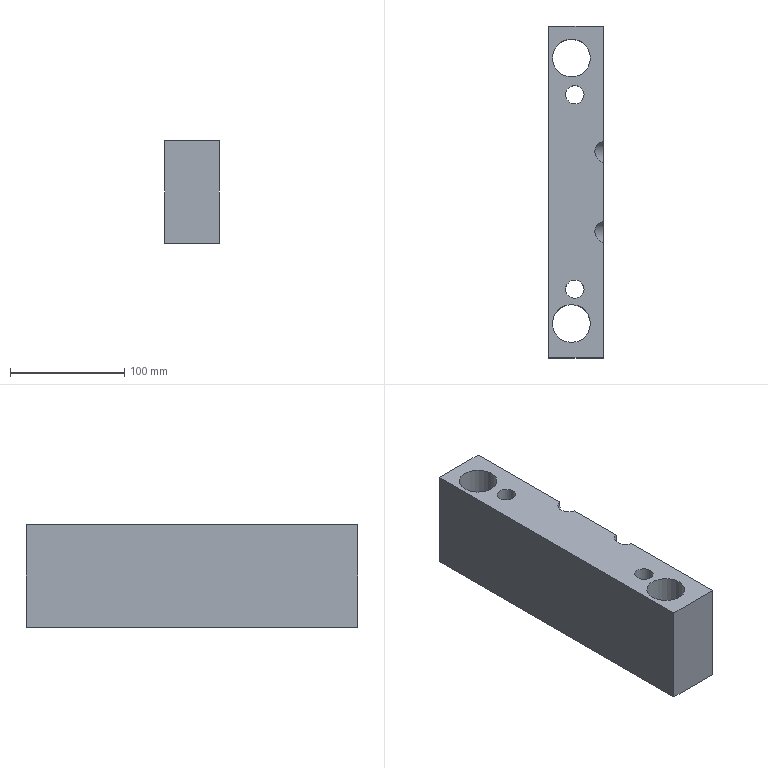Part | STEP file | CC02_id266_x_t | 1 solid | 18 faces | box 48 x 290 x 90 mm | volume 1057434 mm3 | plane 8 | cylinder 8 | cone 2 | commonest cylinder face diameters 10 x2 16 x2 20 x2 33 x2
STEP:
#1=CARTESIAN_POINT('',(113.5,117.,-165.5));
#2=VERTEX_POINT('',#1);
#3=CARTESIAN_POINT('',(97.,117.,-165.5));
#4=DIRECTION('',(0.,0.,1.));
#5=DIRECTION('',(1.,0.,0.));
#6=AXIS2_PLACEMENT_3D('',#3,#4,#5);
#7=CIRCLE('',#6,16.5);
#8=EDGE_CURVE('',#2,#2,#7,.T.);
#9=ORIENTED_EDGE('',*,*,#8,.T.);
#10=EDGE_LOOP('',(#9));
#11=FACE_BOUND('',#10,.T.);
#12=CARTESIAN_POINT('',(95.,-40.,-165.5));
#13=VERTEX_POINT('',#12);
#14=CARTESIAN_POINT('',(100.,-40.,-165.5));
#15=DIRECTION('',(0.,0.,1.));
#16=DIRECTION('',(-1.,0.,0.));
#17=AXIS2_PLACEMENT_3D('',#14,#15,#16);
#18=CIRCLE('',#17,5.);
#19=EDGE_CURVE('',#13,#13,#18,.T.);
#20=ORIENTED_EDGE('',*,*,#19,.T.);
#21=EDGE_LOOP('',(#20));
#22=FACE_BOUND('',#21,.T.);
#23=CARTESIAN_POINT('',(92.,-85.,-165.5));
#24=VERTEX_POINT('',#23);
#25=CARTESIAN_POINT('',(100.,-85.,-165.5));
#26=DIRECTION('',(0.,0.,1.));
#27=DIRECTION('',(-1.,0.,0.));
#28=AXIS2_PLACEMENT_3D('',#25,#26,#27);
#29=CIRCLE('',#28,8.);
#30=EDGE_CURVE('',#24,#24,#29,.T.);
#31=ORIENTED_EDGE('',*,*,#30,.T.);
#32=EDGE_LOOP('',(#31));
#33=FACE_BOUND('',#32,.T.);
#34=CARTESIAN_POINT('',(77.,145.,-165.5));
#35=VERTEX_POINT('',#34);
#36=CARTESIAN_POINT('',(77.,-145.,-165.5));
#37=VERTEX_POINT('',#36);
#38=CARTESIAN_POINT('',(77.,0.,-165.5));
#39=DIRECTION('',(0.,-1.,0.));
#40=VECTOR('',#39,1.);
#41=LINE('',#38,#40);
#42=EDGE_CURVE('',#35,#37,#41,.T.);
#43=ORIENTED_EDGE('',*,*,#42,.F.);
#44=CARTESIAN_POINT('',(125.,145.,-165.5));
#45=VERTEX_POINT('',#44);
#46=CARTESIAN_POINT('',(101.,145.,-165.5));
#47=DIRECTION('',(-1.,0.,0.));
#48=VECTOR('',#47,1.);
#49=LINE('',#46,#48);
#50=EDGE_CURVE('',#45,#35,#49,.T.);
#51=ORIENTED_EDGE('',*,*,#50,.F.);
#52=CARTESIAN_POINT('',(125.,-145.,-165.5));
#53=VERTEX_POINT('',#52);
#54=CARTESIAN_POINT('',(125.,0.,-165.5));
#55=DIRECTION('',(0.,1.,0.));
#56=VECTOR('',#55,1.);
#57=LINE('',#54,#56);
#58=EDGE_CURVE('',#53,#45,#57,.T.);
#59=ORIENTED_EDGE('',*,*,#58,.F.);
#60=CARTESIAN_POINT('',(101.,-145.,-165.5));
#61=DIRECTION('',(1.,0.,0.));
#62=VECTOR('',#61,1.);
#63=LINE('',#60,#62);
#64=EDGE_CURVE('',#37,#53,#63,.T.);
#65=ORIENTED_EDGE('',*,*,#64,.F.);
#66=EDGE_LOOP('',(#43,#51,#59,#65));
#67=FACE_BOUND('',#66,.T.);
#68=CARTESIAN_POINT('',(92.,85.,-165.5));
#69=VERTEX_POINT('',#68);
#70=CARTESIAN_POINT('',(100.,85.,-165.5));
#71=DIRECTION('',(0.,0.,1.));
#72=DIRECTION('',(-1.,0.,0.));
#73=AXIS2_PLACEMENT_3D('',#70,#71,#72);
#74=CIRCLE('',#73,8.);
#75=EDGE_CURVE('',#69,#69,#74,.T.);
#76=ORIENTED_EDGE('',*,*,#75,.T.);
#77=EDGE_LOOP('',(#76));
#78=FACE_BOUND('',#77,.T.);
#79=CARTESIAN_POINT('',(95.,40.,-165.5));
#80=VERTEX_POINT('',#79);
#81=CARTESIAN_POINT('',(100.,40.,-165.5));
#82=DIRECTION('',(0.,0.,1.));
#83=DIRECTION('',(-1.,0.,0.));
#84=AXIS2_PLACEMENT_3D('',#81,#82,#83);
#85=CIRCLE('',#84,5.);
#86=EDGE_CURVE('',#80,#80,#85,.T.);
#87=ORIENTED_EDGE('',*,*,#86,.T.);
#88=EDGE_LOOP('',(#87));
#89=FACE_BOUND('',#88,.T.);
#90=CARTESIAN_POINT('',(113.5,-115.,-165.5));
#91=VERTEX_POINT('',#90);
#92=CARTESIAN_POINT('',(97.,-115.,-165.5));
#93=DIRECTION('',(0.,0.,1.));
#94=DIRECTION('',(1.,0.,0.));
#95=AXIS2_PLACEMENT_3D('',#92,#93,#94);
#96=CIRCLE('',#95,16.5);
#97=EDGE_CURVE('',#91,#91,#96,.T.);
#98=ORIENTED_EDGE('',*,*,#97,.T.);
#99=EDGE_LOOP('',(#98));
#100=FACE_BOUND('',#99,.T.);
#101=CARTESIAN_POINT('',(101.,0.,-165.5));
#102=DIRECTION('',(0.,0.,-1.));
#103=DIRECTION('',(1.,0.,0.));
#104=AXIS2_PLACEMENT_3D('',#101,#102,#103);
#105=PLANE('',#104);
#106=ADVANCED_FACE('',(#11,#22,#33,#67,#78,#89,#100),#105,.T.);
#107=CARTESIAN_POINT('',(125.,-25.437,-75.5));
#108=VERTEX_POINT('',#107);
#109=CARTESIAN_POINT('',(125.,-44.563,-75.5));
#110=VERTEX_POINT('',#109);
#111=CARTESIAN_POINT('',(128.112,-35.,-75.5));
#112=DIRECTION('',(0.,0.,1.));
#113=DIRECTION('',(-1.,0.,0.));
#114=AXIS2_PLACEMENT_3D('',#111,#112,#113);
#115=ELLIPSE('',#114,10.642,10.);
#116=EDGE_CURVE('',#108,#110,#115,.T.);
#117=ORIENTED_EDGE('',*,*,#116,.F.);
#118=CARTESIAN_POINT('',(125.,25.437,-75.5));
#119=VERTEX_POINT('',#118);
#120=CARTESIAN_POINT('',(125.,0.,-75.5));
#121=DIRECTION('',(0.,-1.,0.));
#122=VECTOR('',#121,1.);
#123=LINE('',#120,#122);
#124=EDGE_CURVE('',#119,#108,#123,.T.);
#125=ORIENTED_EDGE('',*,*,#124,.F.);
#126=CARTESIAN_POINT('',(125.,44.563,-75.5));
#127=VERTEX_POINT('',#126);
#128=CARTESIAN_POINT('',(128.112,35.,-75.5));
#129=DIRECTION('',(0.,0.,1.));
#130=DIRECTION('',(-1.,0.,0.));
#131=AXIS2_PLACEMENT_3D('',#128,#129,#130);
#132=ELLIPSE('',#131,10.642,10.);
#133=EDGE_CURVE('',#127,#119,#132,.T.);
#134=ORIENTED_EDGE('',*,*,#133,.F.);
#135=CARTESIAN_POINT('',(125.,145.,-75.5));
#136=VERTEX_POINT('',#135);
#137=CARTESIAN_POINT('',(125.,0.,-75.5));
#138=DIRECTION('',(0.,-1.,0.));
#139=VECTOR('',#138,1.);
#140=LINE('',#137,#139);
#141=EDGE_CURVE('',#136,#127,#140,.T.);
#142=ORIENTED_EDGE('',*,*,#141,.F.);
#143=CARTESIAN_POINT('',(77.,145.,-75.5));
#144=VERTEX_POINT('',#143);
#145=CARTESIAN_POINT('',(101.,145.,-75.5));
#146=DIRECTION('',(1.,0.,0.));
#147=VECTOR('',#146,1.);
#148=LINE('',#145,#147);
#149=EDGE_CURVE('',#144,#136,#148,.T.);
#150=ORIENTED_EDGE('',*,*,#149,.F.);
#151=CARTESIAN_POINT('',(77.,-145.,-75.5));
#152=VERTEX_POINT('',#151);
#153=CARTESIAN_POINT('',(77.,0.,-75.5));
#154=DIRECTION('',(0.,1.,0.));
#155=VECTOR('',#154,1.);
#156=LINE('',#153,#155);
#157=EDGE_CURVE('',#152,#144,#156,.T.);
#158=ORIENTED_EDGE('',*,*,#157,.F.);
#159=CARTESIAN_POINT('',(125.,-145.,-75.5));
#160=VERTEX_POINT('',#159);
#161=CARTESIAN_POINT('',(101.,-145.,-75.5));
#162=DIRECTION('',(-1.,0.,0.));
#163=VECTOR('',#162,1.);
#164=LINE('',#161,#163);
#165=EDGE_CURVE('',#160,#152,#164,.T.);
#166=ORIENTED_EDGE('',*,*,#165,.F.);
#167=CARTESIAN_POINT('',(125.,0.,-75.5));
#168=DIRECTION('',(0.,-1.,0.));
#169=VECTOR('',#168,1.);
#170=LINE('',#167,#169);
#171=EDGE_CURVE('',#110,#160,#170,.T.);
#172=ORIENTED_EDGE('',*,*,#171,.F.);
#173=EDGE_LOOP('',(#117,#125,#134,#142,#150,#158,#166,#172));
#174=FACE_BOUND('',#173,.T.);
#175=CARTESIAN_POINT('',(113.5,117.,-75.5));
#176=VERTEX_POINT('',#175);
#177=CARTESIAN_POINT('',(97.,117.,-75.5));
#178=DIRECTION('',(0.,0.,-1.));
#179=DIRECTION('',(1.,0.,0.));
#180=AXIS2_PLACEMENT_3D('',#177,#178,#179);
#181=CIRCLE('',#180,16.5);
#182=EDGE_CURVE('',#176,#176,#181,.T.);
#183=ORIENTED_EDGE('',*,*,#182,.T.);
#184=EDGE_LOOP('',(#183));
#185=FACE_BOUND('',#184,.T.);
#186=CARTESIAN_POINT('',(108.,-85.,-75.5));
#187=VERTEX_POINT('',#186);
#188=CARTESIAN_POINT('',(100.,-85.,-75.5));
#189=DIRECTION('',(0.,0.,-1.));
#190=DIRECTION('',(1.,0.,0.));
#191=AXIS2_PLACEMENT_3D('',#188,#189,#190);
#192=CIRCLE('',#191,8.);
#193=EDGE_CURVE('',#187,#187,#192,.T.);
#194=ORIENTED_EDGE('',*,*,#193,.T.);
#195=EDGE_LOOP('',(#194));
#196=FACE_BOUND('',#195,.T.);
#197=CARTESIAN_POINT('',(108.,85.,-75.5));
#198=VERTEX_POINT('',#197);
#199=CARTESIAN_POINT('',(100.,85.,-75.5));
#200=DIRECTION('',(0.,0.,-1.));
#201=DIRECTION('',(1.,0.,0.));
#202=AXIS2_PLACEMENT_3D('',#199,#200,#201);
#203=CIRCLE('',#202,8.);
#204=EDGE_CURVE('',#198,#198,#203,.T.);
#205=ORIENTED_EDGE('',*,*,#204,.T.);
#206=EDGE_LOOP('',(#205));
#207=FACE_BOUND('',#206,.T.);
#208=CARTESIAN_POINT('',(113.5,-115.,-75.5));
#209=VERTEX_POINT('',#208);
#210=CARTESIAN_POINT('',(97.,-115.,-75.5));
#211=DIRECTION('',(0.,0.,-1.));
#212=DIRECTION('',(1.,0.,0.));
#213=AXIS2_PLACEMENT_3D('',#210,#211,#212);
#214=CIRCLE('',#213,16.5);
#215=EDGE_CURVE('',#209,#209,#214,.T.);
#216=ORIENTED_EDGE('',*,*,#215,.T.);
#217=EDGE_LOOP('',(#216));
#218=FACE_BOUND('',#217,.T.);
#219=CARTESIAN_POINT('',(101.,0.,-75.5));
#220=DIRECTION('',(0.,0.,1.));
#221=DIRECTION('',(-1.,0.,0.));
#222=AXIS2_PLACEMENT_3D('',#219,#220,#221);
#223=PLANE('',#222);
#224=ADVANCED_FACE('',(#174,#185,#196,#207,#218),#223,.T.);
#225=CARTESIAN_POINT('',(77.,145.,-165.5));
#226=DIRECTION('',(0.,0.,1.));
#227=VECTOR('',#226,1.);
#228=LINE('',#225,#227);
#229=EDGE_CURVE('',#35,#144,#228,.T.);
#230=ORIENTED_EDGE('',*,*,#229,.T.);
#231=ORIENTED_EDGE('',*,*,#149,.T.);
#232=CARTESIAN_POINT('',(125.,145.,-165.5));
#233=DIRECTION('',(0.,0.,1.));
#234=VECTOR('',#233,1.);
#235=LINE('',#232,#234);
#236=EDGE_CURVE('',#45,#136,#235,.T.);
#237=ORIENTED_EDGE('',*,*,#236,.F.);
#238=ORIENTED_EDGE('',*,*,#50,.T.);
#239=EDGE_LOOP('',(#230,#231,#237,#238));
#240=FACE_OUTER_BOUND('',#239,.T.);
#241=CARTESIAN_POINT('',(101.,145.,-165.5));
#242=DIRECTION('',(0.,1.,0.));
#243=DIRECTION('',(0.,0.,-1.));
#244=AXIS2_PLACEMENT_3D('',#241,#242,#243);
#245=PLANE('',#244);
#246=ADVANCED_FACE('',(#240),#245,.T.);
#247=CARTESIAN_POINT('',(125.,-35.,-66.95));
#248=DIRECTION('',(1.,0.,0.));
#249=DIRECTION('',(0.,0.,1.));
#250=AXIS2_PLACEMENT_3D('',#247,#248,#249);
#251=ELLIPSE('',#250,29.238,10.);
#252=EDGE_CURVE('',#110,#108,#251,.T.);
#253=ORIENTED_EDGE('',*,*,#252,.F.);
#254=ORIENTED_EDGE('',*,*,#171,.T.);
#255=CARTESIAN_POINT('',(125.,-145.,-165.5));
#256=DIRECTION('',(0.,0.,1.));
#257=VECTOR('',#256,1.);
#258=LINE('',#255,#257);
#259=EDGE_CURVE('',#53,#160,#258,.T.);
#260=ORIENTED_EDGE('',*,*,#259,.F.);
#261=ORIENTED_EDGE('',*,*,#58,.T.);
#262=ORIENTED_EDGE('',*,*,#236,.T.);
#263=ORIENTED_EDGE('',*,*,#141,.T.);
#264=CARTESIAN_POINT('',(125.,35.,-66.95));
#265=DIRECTION('',(1.,0.,0.));
#266=DIRECTION('',(0.,0.,1.));
#267=AXIS2_PLACEMENT_3D('',#264,#265,#266);
#268=ELLIPSE('',#267,29.238,10.);
#269=EDGE_CURVE('',#119,#127,#268,.T.);
#270=ORIENTED_EDGE('',*,*,#269,.F.);
#271=ORIENTED_EDGE('',*,*,#124,.T.);
#272=EDGE_LOOP('',(#253,#254,#260,#261,#262,#263,#270,#271));
#273=FACE_OUTER_BOUND('',#272,.T.);
#274=CARTESIAN_POINT('',(125.,0.,-165.5));
#275=DIRECTION('',(1.,0.,0.));
#276=DIRECTION('',(0.,0.,1.));
#277=AXIS2_PLACEMENT_3D('',#274,#275,#276);
#278=PLANE('',#277);
#279=ADVANCED_FACE('',(#273),#278,.T.);
#280=ORIENTED_EDGE('',*,*,#259,.T.);
#281=ORIENTED_EDGE('',*,*,#165,.T.);
#282=CARTESIAN_POINT('',(77.,-145.,-165.5));
#283=DIRECTION('',(0.,0.,1.));
#284=VECTOR('',#283,1.);
#285=LINE('',#282,#284);
#286=EDGE_CURVE('',#37,#152,#285,.T.);
#287=ORIENTED_EDGE('',*,*,#286,.F.);
#288=ORIENTED_EDGE('',*,*,#64,.T.);
#289=EDGE_LOOP('',(#280,#281,#287,#288));
#290=FACE_OUTER_BOUND('',#289,.T.);
#291=CARTESIAN_POINT('',(101.,-145.,-165.5));
#292=DIRECTION('',(0.,-1.,0.));
#293=DIRECTION('',(0.,0.,1.));
#294=AXIS2_PLACEMENT_3D('',#291,#292,#293);
#295=PLANE('',#294);
#296=ADVANCED_FACE('',(#290),#295,.T.);
#297=ORIENTED_EDGE('',*,*,#42,.T.);
#298=ORIENTED_EDGE('',*,*,#286,.T.);
#299=ORIENTED_EDGE('',*,*,#157,.T.);
#300=ORIENTED_EDGE('',*,*,#229,.F.);
#301=EDGE_LOOP('',(#297,#298,#299,#300));
#302=FACE_OUTER_BOUND('',#301,.T.);
#303=CARTESIAN_POINT('',(77.,0.,-165.5));
#304=DIRECTION('',(-1.,0.,0.));
#305=DIRECTION('',(0.,0.,-1.));
#306=AXIS2_PLACEMENT_3D('',#303,#304,#305);
#307=PLANE('',#306);
#308=ADVANCED_FACE('',(#302),#307,.T.);
#309=ORIENTED_EDGE('',*,*,#193,.F.);
#310=EDGE_LOOP('',(#309));
#311=FACE_BOUND('',#310,.T.);
#312=ORIENTED_EDGE('',*,*,#30,.F.);
#313=EDGE_LOOP('',(#312));
#314=FACE_BOUND('',#313,.T.);
#315=CARTESIAN_POINT('',(100.,-85.,-165.5));
#316=DIRECTION('',(0.,0.,1.));
#317=DIRECTION('',(-1.,0.,0.));
#318=AXIS2_PLACEMENT_3D('',#315,#316,#317);
#319=CYLINDRICAL_SURFACE('',#318,8.);
#320=ADVANCED_FACE('',(#311,#314),#319,.F.);
#321=ORIENTED_EDGE('',*,*,#204,.F.);
#322=EDGE_LOOP('',(#321));
#323=FACE_BOUND('',#322,.T.);
#324=ORIENTED_EDGE('',*,*,#75,.F.);
#325=EDGE_LOOP('',(#324));
#326=FACE_BOUND('',#325,.T.);
#327=CARTESIAN_POINT('',(100.,85.,-165.5));
#328=DIRECTION('',(0.,0.,1.));
#329=DIRECTION('',(-1.,0.,0.));
#330=AXIS2_PLACEMENT_3D('',#327,#328,#329);
#331=CYLINDRICAL_SURFACE('',#330,8.);
#332=ADVANCED_FACE('',(#323,#326),#331,.F.);
#333=CARTESIAN_POINT('',(95.5,-40.,-144.5));
#334=VERTEX_POINT('',#333);
#335=CARTESIAN_POINT('',(100.,-40.,-144.5));
#336=DIRECTION('',(0.,0.,1.));
#337=DIRECTION('',(-1.,0.,0.));
#338=AXIS2_PLACEMENT_3D('',#335,#336,#337);
#339=CIRCLE('',#338,4.5);
#340=EDGE_CURVE('',#334,#334,#339,.T.);
#341=ORIENTED_EDGE('',*,*,#340,.T.);
#342=EDGE_LOOP('',(#341));
#343=FACE_BOUND('',#342,.T.);
#344=CARTESIAN_POINT('',(105.,-40.,-144.5));
#345=VERTEX_POINT('',#344);
#346=CARTESIAN_POINT('',(100.,-40.,-144.5));
#347=DIRECTION('',(0.,0.,-1.));
#348=DIRECTION('',(1.,0.,0.));
#349=AXIS2_PLACEMENT_3D('',#346,#347,#348);
#350=CIRCLE('',#349,5.);
#351=EDGE_CURVE('',#345,#345,#350,.T.);
#352=ORIENTED_EDGE('',*,*,#351,.T.);
#353=EDGE_LOOP('',(#352));
#354=FACE_BOUND('',#353,.T.);
#355=CARTESIAN_POINT('',(100.,-40.,-144.5));
#356=DIRECTION('',(0.,0.,1.));
#357=DIRECTION('',(-1.,0.,0.));
#358=AXIS2_PLACEMENT_3D('',#355,#356,#357);
#359=PLANE('',#358);
#360=ADVANCED_FACE('',(#343,#354),#359,.F.);
#361=ORIENTED_EDGE('',*,*,#351,.F.);
#362=EDGE_LOOP('',(#361));
#363=FACE_BOUND('',#362,.T.);
#364=ORIENTED_EDGE('',*,*,#19,.F.);
#365=EDGE_LOOP('',(#364));
#366=FACE_BOUND('',#365,.T.);
#367=CARTESIAN_POINT('',(100.,-40.,-165.5));
#368=DIRECTION('',(0.,0.,1.));
#369=DIRECTION('',(-1.,0.,0.));
#370=AXIS2_PLACEMENT_3D('',#367,#368,#369);
#371=CYLINDRICAL_SURFACE('',#370,5.);
#372=ADVANCED_FACE('',(#363,#366),#371,.F.);
#373=CARTESIAN_POINT('',(95.5,40.,-144.5));
#374=VERTEX_POINT('',#373);
#375=CARTESIAN_POINT('',(100.,40.,-144.5));
#376=DIRECTION('',(0.,0.,1.));
#377=DIRECTION('',(-1.,0.,0.));
#378=AXIS2_PLACEMENT_3D('',#375,#376,#377);
#379=CIRCLE('',#378,4.5);
#380=EDGE_CURVE('',#374,#374,#379,.T.);
#381=ORIENTED_EDGE('',*,*,#380,.T.);
#382=EDGE_LOOP('',(#381));
#383=FACE_BOUND('',#382,.T.);
#384=CARTESIAN_POINT('',(105.,40.,-144.5));
#385=VERTEX_POINT('',#384);
#386=CARTESIAN_POINT('',(100.,40.,-144.5));
#387=DIRECTION('',(0.,0.,-1.));
#388=DIRECTION('',(1.,0.,0.));
#389=AXIS2_PLACEMENT_3D('',#386,#387,#388);
#390=CIRCLE('',#389,5.);
#391=EDGE_CURVE('',#385,#385,#390,.T.);
#392=ORIENTED_EDGE('',*,*,#391,.T.);
#393=EDGE_LOOP('',(#392));
#394=FACE_BOUND('',#393,.T.);
#395=CARTESIAN_POINT('',(100.,40.,-144.5));
#396=DIRECTION('',(0.,0.,1.));
#397=DIRECTION('',(-1.,0.,0.));
#398=AXIS2_PLACEMENT_3D('',#395,#396,#397);
#399=PLANE('',#398);
#400=ADVANCED_FACE('',(#383,#394),#399,.F.);
#401=ORIENTED_EDGE('',*,*,#391,.F.);
#402=EDGE_LOOP('',(#401));
#403=FACE_BOUND('',#402,.T.);
#404=ORIENTED_EDGE('',*,*,#86,.F.);
#405=EDGE_LOOP('',(#404));
#406=FACE_BOUND('',#405,.T.);
#407=CARTESIAN_POINT('',(100.,40.,-165.5));
#408=DIRECTION('',(0.,0.,1.));
#409=DIRECTION('',(-1.,0.,0.));
#410=AXIS2_PLACEMENT_3D('',#407,#408,#409);
#411=CYLINDRICAL_SURFACE('',#410,5.);
#412=ADVANCED_FACE('',(#403,#406),#411,.F.);
#413=ORIENTED_EDGE('',*,*,#340,.F.);
#414=EDGE_LOOP('',(#413));
#415=FACE_BOUND('',#414,.T.);
#416=CARTESIAN_POINT('',(100.,-40.,-142.05));
#417=VERTEX_POINT('',#416);
#418=VERTEX_LOOP('',#417);
#419=FACE_BOUND('',#418,.T.);
#420=CARTESIAN_POINT('',(100.,-40.,-142.05));
#421=DIRECTION('',(0.,0.,-1.));
#422=DIRECTION('',(1.,0.,0.));
#423=AXIS2_PLACEMENT_3D('',#420,#421,#422);
#424=CONICAL_SURFACE('',#423,0.,61.434);
#425=ADVANCED_FACE('',(#415,#419),#424,.F.);
#426=ORIENTED_EDGE('',*,*,#380,.F.);
#427=EDGE_LOOP('',(#426));
#428=FACE_BOUND('',#427,.T.);
#429=CARTESIAN_POINT('',(100.,40.,-142.05));
#430=VERTEX_POINT('',#429);
#431=VERTEX_LOOP('',#430);
#432=FACE_BOUND('',#431,.T.);
#433=CARTESIAN_POINT('',(100.,40.,-142.05));
#434=DIRECTION('',(0.,0.,-1.));
#435=DIRECTION('',(1.,0.,0.));
#436=AXIS2_PLACEMENT_3D('',#433,#434,#435);
#437=CONICAL_SURFACE('',#436,0.,61.434);
#438=ADVANCED_FACE('',(#428,#432),#437,.F.);
#439=ORIENTED_EDGE('',*,*,#182,.F.);
#440=EDGE_LOOP('',(#439));
#441=FACE_BOUND('',#440,.T.);
#442=ORIENTED_EDGE('',*,*,#8,.F.);
#443=EDGE_LOOP('',(#442));
#444=FACE_BOUND('',#443,.T.);
#445=CARTESIAN_POINT('',(97.,117.,-165.5));
#446=DIRECTION('',(0.,0.,1.));
#447=DIRECTION('',(1.,0.,0.));
#448=AXIS2_PLACEMENT_3D('',#445,#446,#447);
#449=CYLINDRICAL_SURFACE('',#448,16.5);
#450=ADVANCED_FACE('',(#441,#444),#449,.F.);
#451=ORIENTED_EDGE('',*,*,#215,.F.);
#452=EDGE_LOOP('',(#451));
#453=FACE_BOUND('',#452,.T.);
#454=ORIENTED_EDGE('',*,*,#97,.F.);
#455=EDGE_LOOP('',(#454));
#456=FACE_BOUND('',#455,.T.);
#457=CARTESIAN_POINT('',(97.,-115.,-165.5));
#458=DIRECTION('',(0.,0.,1.));
#459=DIRECTION('',(1.,0.,0.));
#460=AXIS2_PLACEMENT_3D('',#457,#458,#459);
#461=CYLINDRICAL_SURFACE('',#460,16.5);
#462=ADVANCED_FACE('',(#453,#456),#461,.F.);
#463=ORIENTED_EDGE('',*,*,#133,.T.);
#464=ORIENTED_EDGE('',*,*,#269,.T.);
#465=EDGE_LOOP('',(#463,#464));
#466=FACE_OUTER_BOUND('',#465,.T.);
#467=CARTESIAN_POINT('',(105.,35.,-12.));
#468=DIRECTION('',(-0.342,0.,0.9397));
#469=DIRECTION('',(-0.9397,0.,-0.342));
#470=AXIS2_PLACEMENT_3D('',#467,#468,#469);
#471=CYLINDRICAL_SURFACE('',#470,10.);
#472=ADVANCED_FACE('',(#466),#471,.F.);
#473=ORIENTED_EDGE('',*,*,#116,.T.);
#474=ORIENTED_EDGE('',*,*,#252,.T.);
#475=EDGE_LOOP('',(#473,#474));
#476=FACE_OUTER_BOUND('',#475,.T.);
#477=CARTESIAN_POINT('',(105.,-35.,-12.));
#478=DIRECTION('',(-0.342,0.,0.9397));
#479=DIRECTION('',(-0.9397,0.,-0.342));
#480=AXIS2_PLACEMENT_3D('',#477,#478,#479);
#481=CYLINDRICAL_SURFACE('',#480,10.);
#482=ADVANCED_FACE('',(#476),#481,.F.);
#483=CLOSED_SHELL('',(#106,#224,#246,#279,#296,#308,#320,#332,#360,#372,#400,#412,#425,#438,#450,#462,#472,#482));
#484=MANIFOLD_SOLID_BREP('',#483);
#485=(LENGTH_UNIT()NAMED_UNIT(*)SI_UNIT(.MILLI.,.METRE.));
#486=UNCERTAINTY_MEASURE_WITH_UNIT(LENGTH_MEASURE(0.00002),#485,'','');
#487=(NAMED_UNIT(*)PLANE_ANGLE_UNIT()SI_UNIT($,.RADIAN.));
#488=PLANE_ANGLE_MEASURE_WITH_UNIT(PLANE_ANGLE_MEASURE(0.01745),#487);
#489=DIMENSIONAL_EXPONENTS(0.,0.,0.,0.,0.,0.,0.);
#490=(CONVERSION_BASED_UNIT('DEGREE',#488)NAMED_UNIT(#489)PLANE_ANGLE_UNIT());
#491=(NAMED_UNIT(*)SI_UNIT($,.STERADIAN.)SOLID_ANGLE_UNIT());
#492=(GEOMETRIC_REPRESENTATION_CONTEXT(3)GLOBAL_UNCERTAINTY_ASSIGNED_CONTEXT((#486))GLOBAL_UNIT_ASSIGNED_CONTEXT((#485,#490,#491))REPRESENTATION_CONTEXT('',''));
#493=ADVANCED_BREP_SHAPE_REPRESENTATION('',(#484),#492);